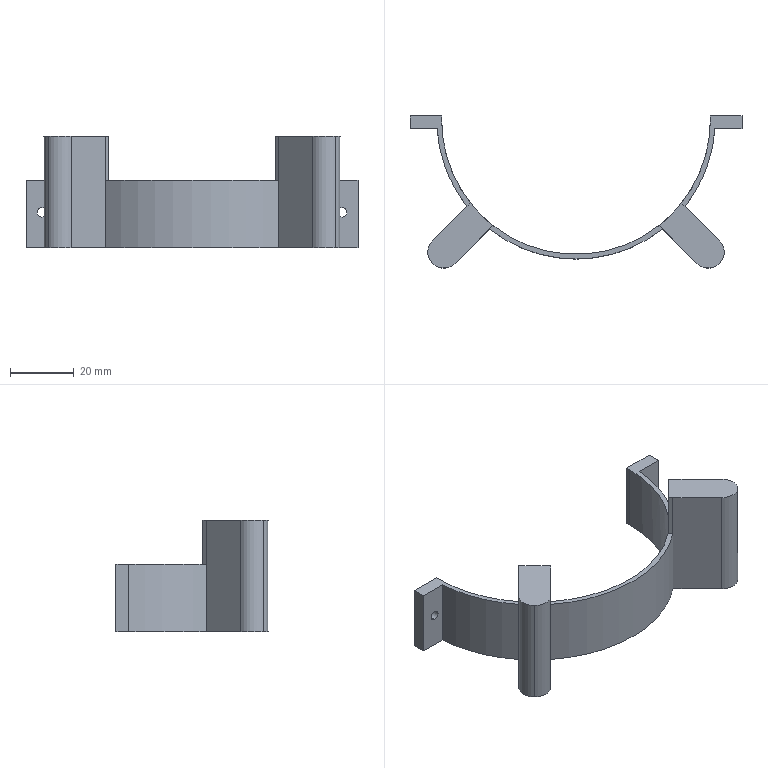Part | SolidWorks | features ICE 8, Fillet 2, CirPattern 1, Extrusion 1 | 1 solid | 40 faces | box 104 x 47.686 x 35 mm | volume 18349 mm3 | plane 22 | cylinder 18 | commonest cylinder face diameters 3 x4 5 x4 10 x4 84.2 x3 87.2 x3
STEP:
#1=CARTESIAN_POINT('',(43.936,-41.436,28.));
#2=VERTEX_POINT('',#1);
#3=CARTESIAN_POINT('',(38.936,-41.436,28.));
#4=VERTEX_POINT('',#3);
#5=CARTESIAN_POINT('',(41.436,-41.436,28.));
#6=DIRECTION('',(0.,0.,-1.));
#7=DIRECTION('',(0.,-1.,0.));
#8=AXIS2_PLACEMENT_3D('',#5,#6,#7);
#9=CIRCLE('',#8,2.5);
#10=EDGE_CURVE('',#2,#4,#9,.T.);
#11=ORIENTED_EDGE('',*,*,#10,.F.);
#12=CARTESIAN_POINT('',(43.936,-41.436,0.));
#13=VERTEX_POINT('',#12);
#14=CARTESIAN_POINT('',(43.936,-41.436,28.));
#15=DIRECTION('',(0.,0.,-1.));
#16=VECTOR('',#15,1000.);
#17=LINE('',#14,#16);
#18=EDGE_CURVE('',#2,#13,#17,.T.);
#19=ORIENTED_EDGE('',*,*,#18,.T.);
#20=CARTESIAN_POINT('',(38.936,-41.436,0.));
#21=VERTEX_POINT('',#20);
#22=CARTESIAN_POINT('',(41.436,-41.436,0.));
#23=DIRECTION('',(0.,0.,-1.));
#24=DIRECTION('',(0.,-1.,0.));
#25=AXIS2_PLACEMENT_3D('',#22,#23,#24);
#26=CIRCLE('',#25,2.5);
#27=EDGE_CURVE('',#13,#21,#26,.T.);
#28=ORIENTED_EDGE('',*,*,#27,.T.);
#29=CARTESIAN_POINT('',(38.936,-41.436,28.));
#30=DIRECTION('',(0.,0.,-1.));
#31=VECTOR('',#30,1000.);
#32=LINE('',#29,#31);
#33=EDGE_CURVE('',#4,#21,#32,.T.);
#34=ORIENTED_EDGE('',*,*,#33,.F.);
#35=EDGE_LOOP('',(#11,#19,#28,#34));
#36=FACE_OUTER_BOUND('',#35,.T.);
#37=CARTESIAN_POINT('',(41.436,-41.436,28.));
#38=DIRECTION('',(0.,0.,-1.));
#39=DIRECTION('',(-1.,0.,0.));
#40=AXIS2_PLACEMENT_3D('',#37,#38,#39);
#41=CYLINDRICAL_SURFACE('',#40,2.5);
#42=ADVANCED_FACE('',(#36),#41,.F.);
#43=CARTESIAN_POINT('',(-38.936,-41.436,28.));
#44=VERTEX_POINT('',#43);
#45=CARTESIAN_POINT('',(-43.936,-41.436,28.));
#46=VERTEX_POINT('',#45);
#47=CARTESIAN_POINT('',(-41.436,-41.436,28.));
#48=DIRECTION('',(0.,0.,-1.));
#49=DIRECTION('',(-1.,0.,0.));
#50=AXIS2_PLACEMENT_3D('',#47,#48,#49);
#51=CIRCLE('',#50,2.5);
#52=EDGE_CURVE('',#44,#46,#51,.T.);
#53=ORIENTED_EDGE('',*,*,#52,.F.);
#54=CARTESIAN_POINT('',(-38.936,-41.436,0.));
#55=VERTEX_POINT('',#54);
#56=CARTESIAN_POINT('',(-38.936,-41.436,28.));
#57=DIRECTION('',(0.,0.,-1.));
#58=VECTOR('',#57,1000.);
#59=LINE('',#56,#58);
#60=EDGE_CURVE('',#44,#55,#59,.T.);
#61=ORIENTED_EDGE('',*,*,#60,.T.);
#62=CARTESIAN_POINT('',(-43.936,-41.436,0.));
#63=VERTEX_POINT('',#62);
#64=CARTESIAN_POINT('',(-41.436,-41.436,0.));
#65=DIRECTION('',(0.,0.,-1.));
#66=DIRECTION('',(-1.,0.,0.));
#67=AXIS2_PLACEMENT_3D('',#64,#65,#66);
#68=CIRCLE('',#67,2.5);
#69=EDGE_CURVE('',#55,#63,#68,.T.);
#70=ORIENTED_EDGE('',*,*,#69,.T.);
#71=CARTESIAN_POINT('',(-43.936,-41.436,28.));
#72=DIRECTION('',(0.,0.,-1.));
#73=VECTOR('',#72,1000.);
#74=LINE('',#71,#73);
#75=EDGE_CURVE('',#46,#63,#74,.T.);
#76=ORIENTED_EDGE('',*,*,#75,.F.);
#77=EDGE_LOOP('',(#53,#61,#70,#76));
#78=FACE_OUTER_BOUND('',#77,.T.);
#79=CARTESIAN_POINT('',(-41.436,-41.436,28.));
#80=DIRECTION('',(0.,0.,-1.));
#81=DIRECTION('',(-1.,0.,0.));
#82=AXIS2_PLACEMENT_3D('',#79,#80,#81);
#83=CYLINDRICAL_SURFACE('',#82,2.5);
#84=ADVANCED_FACE('',(#78),#83,.F.);
#85=CARTESIAN_POINT('',(47.001,-2.75,9.64));
#86=VERTEX_POINT('',#85);
#87=CARTESIAN_POINT('',(47.001,-2.75,12.64));
#88=VERTEX_POINT('',#87);
#89=CARTESIAN_POINT('',(47.001,-2.75,11.14));
#90=DIRECTION('',(0.,1.,0.));
#91=DIRECTION('',(0.,0.,-1.));
#92=AXIS2_PLACEMENT_3D('',#89,#90,#91);
#93=CIRCLE('',#92,1.5);
#94=EDGE_CURVE('',#86,#88,#93,.T.);
#95=ORIENTED_EDGE('',*,*,#94,.F.);
#96=CARTESIAN_POINT('',(47.001,1.25,9.64));
#97=VERTEX_POINT('',#96);
#98=CARTESIAN_POINT('',(47.001,-43.601,9.64));
#99=DIRECTION('',(0.,1.,0.));
#100=VECTOR('',#99,1000.);
#101=LINE('',#98,#100);
#102=EDGE_CURVE('',#86,#97,#101,.T.);
#103=ORIENTED_EDGE('',*,*,#102,.T.);
#104=CARTESIAN_POINT('',(47.001,1.25,12.64));
#105=VERTEX_POINT('',#104);
#106=CARTESIAN_POINT('',(47.001,1.25,11.14));
#107=DIRECTION('',(0.,1.,0.));
#108=DIRECTION('',(0.,0.,1.));
#109=AXIS2_PLACEMENT_3D('',#106,#107,#108);
#110=CIRCLE('',#109,1.5);
#111=EDGE_CURVE('',#97,#105,#110,.T.);
#112=ORIENTED_EDGE('',*,*,#111,.T.);
#113=CARTESIAN_POINT('',(47.001,-43.601,12.64));
#114=DIRECTION('',(0.,1.,0.));
#115=VECTOR('',#114,1000.);
#116=LINE('',#113,#115);
#117=EDGE_CURVE('',#88,#105,#116,.T.);
#118=ORIENTED_EDGE('',*,*,#117,.F.);
#119=EDGE_LOOP('',(#95,#103,#112,#118));
#120=FACE_OUTER_BOUND('',#119,.T.);
#121=CARTESIAN_POINT('',(47.001,-43.601,11.14));
#122=DIRECTION('',(0.,1.,0.));
#123=DIRECTION('',(0.,0.,1.));
#124=AXIS2_PLACEMENT_3D('',#121,#122,#123);
#125=CYLINDRICAL_SURFACE('',#124,1.5);
#126=ADVANCED_FACE('',(#120),#125,.F.);
#127=CARTESIAN_POINT('',(-47.001,-2.75,12.64));
#128=VERTEX_POINT('',#127);
#129=CARTESIAN_POINT('',(-47.001,-2.75,9.64));
#130=VERTEX_POINT('',#129);
#131=CARTESIAN_POINT('',(-47.001,-2.75,11.14));
#132=DIRECTION('',(0.,-1.,0.));
#133=DIRECTION('',(0.,0.,1.));
#134=AXIS2_PLACEMENT_3D('',#131,#132,#133);
#135=CIRCLE('',#134,1.5);
#136=EDGE_CURVE('',#128,#130,#135,.T.);
#137=ORIENTED_EDGE('',*,*,#136,.T.);
#138=CARTESIAN_POINT('',(-47.001,1.25,9.64));
#139=VERTEX_POINT('',#138);
#140=CARTESIAN_POINT('',(-47.001,-43.601,9.64));
#141=DIRECTION('',(0.,1.,0.));
#142=VECTOR('',#141,1000.);
#143=LINE('',#140,#142);
#144=EDGE_CURVE('',#130,#139,#143,.T.);
#145=ORIENTED_EDGE('',*,*,#144,.T.);
#146=CARTESIAN_POINT('',(-47.001,1.25,12.64));
#147=VERTEX_POINT('',#146);
#148=CARTESIAN_POINT('',(-47.001,1.25,11.14));
#149=DIRECTION('',(0.,1.,0.));
#150=DIRECTION('',(0.,0.,1.));
#151=AXIS2_PLACEMENT_3D('',#148,#149,#150);
#152=CIRCLE('',#151,1.5);
#153=EDGE_CURVE('',#139,#147,#152,.T.);
#154=ORIENTED_EDGE('',*,*,#153,.T.);
#155=CARTESIAN_POINT('',(-47.001,-43.601,12.64));
#156=DIRECTION('',(0.,1.,0.));
#157=VECTOR('',#156,1000.);
#158=LINE('',#155,#157);
#159=EDGE_CURVE('',#128,#147,#158,.T.);
#160=ORIENTED_EDGE('',*,*,#159,.F.);
#161=EDGE_LOOP('',(#137,#145,#154,#160));
#162=FACE_OUTER_BOUND('',#161,.T.);
#163=CARTESIAN_POINT('',(-47.001,-43.601,11.14));
#164=DIRECTION('',(0.,1.,0.));
#165=DIRECTION('',(0.,0.,1.));
#166=AXIS2_PLACEMENT_3D('',#163,#164,#165);
#167=CYLINDRICAL_SURFACE('',#166,1.5);
#168=ADVANCED_FACE('',(#162),#167,.F.);
#169=CARTESIAN_POINT('',(33.094,-26.023,21.14));
#170=VERTEX_POINT('',#169);
#171=CARTESIAN_POINT('',(42.1,0.,21.14));
#172=VERTEX_POINT('',#171);
#173=CARTESIAN_POINT('',(0.,0.,21.14));
#174=DIRECTION('',(0.,0.,1.));
#175=DIRECTION('',(1.,0.,0.));
#176=AXIS2_PLACEMENT_3D('',#173,#174,#175);
#177=CIRCLE('',#176,42.1);
#178=EDGE_CURVE('',#170,#172,#177,.T.);
#179=ORIENTED_EDGE('',*,*,#178,.T.);
#180=CARTESIAN_POINT('',(42.1,0.,0.));
#181=VERTEX_POINT('',#180);
#182=CARTESIAN_POINT('',(42.1,0.,21.14));
#183=DIRECTION('',(0.,0.,-1.));
#184=VECTOR('',#183,1000.);
#185=LINE('',#182,#184);
#186=EDGE_CURVE('',#172,#181,#185,.T.);
#187=ORIENTED_EDGE('',*,*,#186,.T.);
#188=CARTESIAN_POINT('',(-42.1,0.,0.));
#189=VERTEX_POINT('',#188);
#190=CARTESIAN_POINT('',(0.,0.,0.));
#191=DIRECTION('',(0.,0.,1.));
#192=DIRECTION('',(1.,0.,0.));
#193=AXIS2_PLACEMENT_3D('',#190,#191,#192);
#194=CIRCLE('',#193,42.1);
#195=EDGE_CURVE('',#189,#181,#194,.T.);
#196=ORIENTED_EDGE('',*,*,#195,.F.);
#197=CARTESIAN_POINT('',(-42.1,0.,21.14));
#198=VERTEX_POINT('',#197);
#199=CARTESIAN_POINT('',(-42.1,0.,21.14));
#200=DIRECTION('',(0.,0.,-1.));
#201=VECTOR('',#200,1000.);
#202=LINE('',#199,#201);
#203=EDGE_CURVE('',#198,#189,#202,.T.);
#204=ORIENTED_EDGE('',*,*,#203,.F.);
#205=CARTESIAN_POINT('',(-33.098,-26.018,21.14));
#206=VERTEX_POINT('',#205);
#207=CARTESIAN_POINT('',(0.,0.,21.14));
#208=DIRECTION('',(0.,0.,1.));
#209=DIRECTION('',(1.,0.,0.));
#210=AXIS2_PLACEMENT_3D('',#207,#208,#209);
#211=CIRCLE('',#210,42.1);
#212=EDGE_CURVE('',#198,#206,#211,.T.);
#213=ORIENTED_EDGE('',*,*,#212,.T.);
#214=CARTESIAN_POINT('',(-33.098,-26.018,35.));
#215=VERTEX_POINT('',#214);
#216=CARTESIAN_POINT('',(-33.098,-26.018,35.));
#217=DIRECTION('',(0.,0.,-1.));
#218=VECTOR('',#217,1000.);
#219=LINE('',#216,#218);
#220=EDGE_CURVE('',#215,#206,#219,.T.);
#221=ORIENTED_EDGE('',*,*,#220,.F.);
#222=CARTESIAN_POINT('',(-26.023,-33.094,35.));
#223=VERTEX_POINT('',#222);
#224=CARTESIAN_POINT('',(0.,0.,35.));
#225=DIRECTION('',(0.,0.,-1.));
#226=DIRECTION('',(1.,0.,0.));
#227=AXIS2_PLACEMENT_3D('',#224,#225,#226);
#228=CIRCLE('',#227,42.1);
#229=EDGE_CURVE('',#223,#215,#228,.T.);
#230=ORIENTED_EDGE('',*,*,#229,.F.);
#231=CARTESIAN_POINT('',(-26.023,-33.094,21.14));
#232=VERTEX_POINT('',#231);
#233=CARTESIAN_POINT('',(-26.023,-33.094,35.));
#234=DIRECTION('',(0.,0.,-1.));
#235=VECTOR('',#234,1000.);
#236=LINE('',#233,#235);
#237=EDGE_CURVE('',#223,#232,#236,.T.);
#238=ORIENTED_EDGE('',*,*,#237,.T.);
#239=CARTESIAN_POINT('',(26.018,-33.098,21.14));
#240=VERTEX_POINT('',#239);
#241=CARTESIAN_POINT('',(0.,0.,21.14));
#242=DIRECTION('',(0.,0.,1.));
#243=DIRECTION('',(1.,0.,0.));
#244=AXIS2_PLACEMENT_3D('',#241,#242,#243);
#245=CIRCLE('',#244,42.1);
#246=EDGE_CURVE('',#232,#240,#245,.T.);
#247=ORIENTED_EDGE('',*,*,#246,.T.);
#248=CARTESIAN_POINT('',(26.018,-33.098,35.));
#249=VERTEX_POINT('',#248);
#250=CARTESIAN_POINT('',(26.018,-33.098,35.));
#251=DIRECTION('',(0.,0.,-1.));
#252=VECTOR('',#251,1000.);
#253=LINE('',#250,#252);
#254=EDGE_CURVE('',#249,#240,#253,.T.);
#255=ORIENTED_EDGE('',*,*,#254,.F.);
#256=CARTESIAN_POINT('',(33.094,-26.023,35.));
#257=VERTEX_POINT('',#256);
#258=CARTESIAN_POINT('',(0.,0.,35.));
#259=DIRECTION('',(0.,0.,-1.));
#260=DIRECTION('',(0.,1.,0.));
#261=AXIS2_PLACEMENT_3D('',#258,#259,#260);
#262=CIRCLE('',#261,42.1);
#263=EDGE_CURVE('',#257,#249,#262,.T.);
#264=ORIENTED_EDGE('',*,*,#263,.F.);
#265=CARTESIAN_POINT('',(33.094,-26.023,35.));
#266=DIRECTION('',(0.,0.,-1.));
#267=VECTOR('',#266,1000.);
#268=LINE('',#265,#267);
#269=EDGE_CURVE('',#257,#170,#268,.T.);
#270=ORIENTED_EDGE('',*,*,#269,.T.);
#271=EDGE_LOOP('',(#179,#187,#196,#204,#213,#221,#230,#238,#247,#255,#264,#270));
#272=FACE_OUTER_BOUND('',#271,.T.);
#273=CARTESIAN_POINT('',(0.,0.,21.14));
#274=DIRECTION('',(0.,0.,-1.));
#275=DIRECTION('',(-1.,0.,0.));
#276=AXIS2_PLACEMENT_3D('',#273,#274,#275);
#277=CYLINDRICAL_SURFACE('',#276,42.1);
#278=ADVANCED_FACE('',(#272),#277,.F.);
#279=CARTESIAN_POINT('',(-42.081,1.25,21.14));
#280=VERTEX_POINT('',#279);
#281=CARTESIAN_POINT('',(0.,0.,21.14));
#282=DIRECTION('',(0.,0.,1.));
#283=DIRECTION('',(1.,0.,0.));
#284=AXIS2_PLACEMENT_3D('',#281,#282,#283);
#285=CIRCLE('',#284,42.1);
#286=EDGE_CURVE('',#280,#198,#285,.T.);
#287=ORIENTED_EDGE('',*,*,#286,.T.);
#288=ORIENTED_EDGE('',*,*,#203,.T.);
#289=CARTESIAN_POINT('',(-42.081,1.25,0.));
#290=VERTEX_POINT('',#289);
#291=CARTESIAN_POINT('',(0.,0.,0.));
#292=DIRECTION('',(0.,0.,1.));
#293=DIRECTION('',(1.,0.,0.));
#294=AXIS2_PLACEMENT_3D('',#291,#292,#293);
#295=CIRCLE('',#294,42.1);
#296=EDGE_CURVE('',#290,#189,#295,.T.);
#297=ORIENTED_EDGE('',*,*,#296,.F.);
#298=CARTESIAN_POINT('',(-42.081,1.25,21.14));
#299=DIRECTION('',(0.,0.,-1.));
#300=VECTOR('',#299,1000.);
#301=LINE('',#298,#300);
#302=EDGE_CURVE('',#280,#290,#301,.T.);
#303=ORIENTED_EDGE('',*,*,#302,.F.);
#304=EDGE_LOOP('',(#287,#288,#297,#303));
#305=FACE_OUTER_BOUND('',#304,.T.);
#306=CARTESIAN_POINT('',(0.,0.,21.14));
#307=DIRECTION('',(0.,0.,-1.));
#308=DIRECTION('',(-1.,0.,0.));
#309=AXIS2_PLACEMENT_3D('',#306,#307,#308);
#310=CYLINDRICAL_SURFACE('',#309,42.1);
#311=ADVANCED_FACE('',(#305),#310,.F.);
#312=CARTESIAN_POINT('',(-27.091,-34.162,21.14));
#313=VERTEX_POINT('',#312);
#314=CARTESIAN_POINT('',(27.091,-34.162,21.14));
#315=VERTEX_POINT('',#314);
#316=CARTESIAN_POINT('',(0.,0.,21.14));
#317=DIRECTION('',(0.,0.,1.));
#318=DIRECTION('',(1.,0.,0.));
#319=AXIS2_PLACEMENT_3D('',#316,#317,#318);
#320=CIRCLE('',#319,43.6);
#321=EDGE_CURVE('',#313,#315,#320,.T.);
#322=ORIENTED_EDGE('',*,*,#321,.T.);
#323=CARTESIAN_POINT('',(26.018,-33.098,21.14));
#324=DIRECTION('',(0.7098,-0.7044,0.));
#325=VECTOR('',#324,1000.);
#326=LINE('',#323,#325);
#327=EDGE_CURVE('',#240,#315,#326,.T.);
#328=ORIENTED_EDGE('',*,*,#327,.F.);
#329=ORIENTED_EDGE('',*,*,#246,.F.);
#330=CARTESIAN_POINT('',(-26.023,-33.094,21.14));
#331=DIRECTION('',(0.7068,0.7074,0.));
#332=VECTOR('',#331,1000.);
#333=LINE('',#330,#332);
#334=EDGE_CURVE('',#313,#232,#333,.T.);
#335=ORIENTED_EDGE('',*,*,#334,.F.);
#336=EDGE_LOOP('',(#322,#328,#329,#335));
#337=FACE_OUTER_BOUND('',#336,.T.);
#338=CARTESIAN_POINT('',(0.,0.,21.14));
#339=DIRECTION('',(0.,0.,1.));
#340=DIRECTION('',(1.,0.,0.));
#341=AXIS2_PLACEMENT_3D('',#338,#339,#340);
#342=PLANE('',#341);
#343=ADVANCED_FACE('',(#337),#342,.T.);
#344=ORIENTED_EDGE('',*,*,#178,.F.);
#345=CARTESIAN_POINT('',(34.162,-27.091,21.14));
#346=VERTEX_POINT('',#345);
#347=CARTESIAN_POINT('',(33.094,-26.023,21.14));
#348=DIRECTION('',(-0.7074,0.7068,0.));
#349=VECTOR('',#348,1000.);
#350=LINE('',#347,#349);
#351=EDGE_CURVE('',#346,#170,#350,.T.);
#352=ORIENTED_EDGE('',*,*,#351,.F.);
#353=CARTESIAN_POINT('',(43.513,-2.75,21.14));
#354=VERTEX_POINT('',#353);
#355=CARTESIAN_POINT('',(0.,0.,21.14));
#356=DIRECTION('',(0.,0.,1.));
#357=DIRECTION('',(1.,0.,0.));
#358=AXIS2_PLACEMENT_3D('',#355,#356,#357);
#359=CIRCLE('',#358,43.6);
#360=EDGE_CURVE('',#346,#354,#359,.T.);
#361=ORIENTED_EDGE('',*,*,#360,.T.);
#362=CARTESIAN_POINT('',(52.,-2.75,21.14));
#363=VERTEX_POINT('',#362);
#364=CARTESIAN_POINT('',(-52.002,-2.75,21.14));
#365=DIRECTION('',(1.,0.,0.));
#366=VECTOR('',#365,1000.);
#367=LINE('',#364,#366);
#368=EDGE_CURVE('',#354,#363,#367,.T.);
#369=ORIENTED_EDGE('',*,*,#368,.T.);
#370=CARTESIAN_POINT('',(52.,1.25,21.14));
#371=VERTEX_POINT('',#370);
#372=CARTESIAN_POINT('',(52.,1.25,21.14));
#373=DIRECTION('',(0.,-1.,0.));
#374=VECTOR('',#373,1000.);
#375=LINE('',#372,#374);
#376=EDGE_CURVE('',#371,#363,#375,.T.);
#377=ORIENTED_EDGE('',*,*,#376,.F.);
#378=CARTESIAN_POINT('',(42.081,1.25,21.14));
#379=VERTEX_POINT('',#378);
#380=CARTESIAN_POINT('',(0.,1.25,21.14));
#381=DIRECTION('',(1.,0.,0.));
#382=VECTOR('',#381,1000.);
#383=LINE('',#380,#382);
#384=EDGE_CURVE('',#379,#371,#383,.T.);
#385=ORIENTED_EDGE('',*,*,#384,.F.);
#386=CARTESIAN_POINT('',(0.,0.,21.14));
#387=DIRECTION('',(0.,0.,1.));
#388=DIRECTION('',(1.,0.,0.));
#389=AXIS2_PLACEMENT_3D('',#386,#387,#388);
#390=CIRCLE('',#389,42.1);
#391=EDGE_CURVE('',#172,#379,#390,.T.);
#392=ORIENTED_EDGE('',*,*,#391,.F.);
#393=EDGE_LOOP('',(#344,#352,#361,#369,#377,#385,#392));
#394=FACE_OUTER_BOUND('',#393,.T.);
#395=CARTESIAN_POINT('',(0.,0.,21.14));
#396=DIRECTION('',(0.,0.,1.));
#397=DIRECTION('',(1.,0.,0.));
#398=AXIS2_PLACEMENT_3D('',#395,#396,#397);
#399=PLANE('',#398);
#400=ADVANCED_FACE('',(#394),#399,.T.);
#401=CARTESIAN_POINT('',(27.091,-34.162,0.));
#402=VERTEX_POINT('',#401);
#403=CARTESIAN_POINT('',(27.091,-34.162,21.14));
#404=DIRECTION('',(0.,0.,1.));
#405=VECTOR('',#404,1000.);
#406=LINE('',#403,#405);
#407=EDGE_CURVE('',#402,#315,#406,.T.);
#408=ORIENTED_EDGE('',*,*,#407,.T.);
#409=ORIENTED_EDGE('',*,*,#321,.F.);
#410=CARTESIAN_POINT('',(-27.091,-34.162,0.));
#411=VERTEX_POINT('',#410);
#412=CARTESIAN_POINT('',(-27.091,-34.162,21.14));
#413=DIRECTION('',(0.,0.,-1.));
#414=VECTOR('',#413,1000.);
#415=LINE('',#412,#414);
#416=EDGE_CURVE('',#313,#411,#415,.T.);
#417=ORIENTED_EDGE('',*,*,#416,.T.);
#418=CARTESIAN_POINT('',(0.,0.,0.));
#419=DIRECTION('',(0.,0.,1.));
#420=DIRECTION('',(1.,0.,0.));
#421=AXIS2_PLACEMENT_3D('',#418,#419,#420);
#422=CIRCLE('',#421,43.6);
#423=EDGE_CURVE('',#411,#402,#422,.T.);
#424=ORIENTED_EDGE('',*,*,#423,.T.);
#425=EDGE_LOOP('',(#408,#409,#417,#424));
#426=FACE_OUTER_BOUND('',#425,.T.);
#427=CARTESIAN_POINT('',(0.,0.,21.14));
#428=DIRECTION('',(0.,0.,-1.));
#429=DIRECTION('',(-1.,0.,0.));
#430=AXIS2_PLACEMENT_3D('',#427,#428,#429);
#431=CYLINDRICAL_SURFACE('',#430,43.6);
#432=ADVANCED_FACE('',(#426),#431,.T.);
#433=CARTESIAN_POINT('',(34.162,-27.091,0.));
#434=VERTEX_POINT('',#433);
#435=CARTESIAN_POINT('',(34.162,-27.091,21.14));
#436=DIRECTION('',(0.,0.,-1.));
#437=VECTOR('',#436,1000.);
#438=LINE('',#435,#437);
#439=EDGE_CURVE('',#346,#434,#438,.T.);
#440=ORIENTED_EDGE('',*,*,#439,.T.);
#441=CARTESIAN_POINT('',(43.513,-2.75,0.));
#442=VERTEX_POINT('',#441);
#443=CARTESIAN_POINT('',(0.,0.,0.));
#444=DIRECTION('',(0.,0.,1.));
#445=DIRECTION('',(1.,0.,0.));
#446=AXIS2_PLACEMENT_3D('',#443,#444,#445);
#447=CIRCLE('',#446,43.6);
#448=EDGE_CURVE('',#434,#442,#447,.T.);
#449=ORIENTED_EDGE('',*,*,#448,.T.);
#450=CARTESIAN_POINT('',(43.513,-2.75,21.14));
#451=DIRECTION('',(0.,0.,-1.));
#452=VECTOR('',#451,1000.);
#453=LINE('',#450,#452);
#454=EDGE_CURVE('',#354,#442,#453,.T.);
#455=ORIENTED_EDGE('',*,*,#454,.F.);
#456=ORIENTED_EDGE('',*,*,#360,.F.);
#457=EDGE_LOOP('',(#440,#449,#455,#456));
#458=FACE_OUTER_BOUND('',#457,.T.);
#459=CARTESIAN_POINT('',(0.,0.,21.14));
#460=DIRECTION('',(0.,0.,-1.));
#461=DIRECTION('',(-1.,0.,0.));
#462=AXIS2_PLACEMENT_3D('',#459,#460,#461);
#463=CYLINDRICAL_SURFACE('',#462,43.6);
#464=ADVANCED_FACE('',(#458),#463,.T.);
#465=CARTESIAN_POINT('',(-34.162,-27.091,0.));
#466=VERTEX_POINT('',#465);
#467=CARTESIAN_POINT('',(-34.162,-27.091,21.14));
#468=VERTEX_POINT('',#467);
#469=CARTESIAN_POINT('',(-34.162,-27.091,21.14));
#470=DIRECTION('',(0.,0.,1.));
#471=VECTOR('',#470,1000.);
#472=LINE('',#469,#471);
#473=EDGE_CURVE('',#466,#468,#472,.T.);
#474=ORIENTED_EDGE('',*,*,#473,.T.);
#475=CARTESIAN_POINT('',(-43.513,-2.75,21.14));
#476=VERTEX_POINT('',#475);
#477=CARTESIAN_POINT('',(0.,0.,21.14));
#478=DIRECTION('',(0.,0.,1.));
#479=DIRECTION('',(1.,0.,0.));
#480=AXIS2_PLACEMENT_3D('',#477,#478,#479);
#481=CIRCLE('',#480,43.6);
#482=EDGE_CURVE('',#476,#468,#481,.T.);
#483=ORIENTED_EDGE('',*,*,#482,.F.);
#484=CARTESIAN_POINT('',(-43.513,-2.75,0.));
#485=VERTEX_POINT('',#484);
#486=CARTESIAN_POINT('',(-43.513,-2.75,21.14));
#487=DIRECTION('',(0.,0.,-1.));
#488=VECTOR('',#487,1000.);
#489=LINE('',#486,#488);
#490=EDGE_CURVE('',#476,#485,#489,.T.);
#491=ORIENTED_EDGE('',*,*,#490,.T.);
#492=CARTESIAN_POINT('',(0.,0.,0.));
#493=DIRECTION('',(0.,0.,1.));
#494=DIRECTION('',(1.,0.,0.));
#495=AXIS2_PLACEMENT_3D('',#492,#493,#494);
#496=CIRCLE('',#495,43.6);
#497=EDGE_CURVE('',#485,#466,#496,.T.);
#498=ORIENTED_EDGE('',*,*,#497,.T.);
#499=EDGE_LOOP('',(#474,#483,#491,#498));
#500=FACE_OUTER_BOUND('',#499,.T.);
#501=CARTESIAN_POINT('',(0.,0.,21.14));
#502=DIRECTION('',(0.,0.,-1.));
#503=DIRECTION('',(-1.,0.,0.));
#504=AXIS2_PLACEMENT_3D('',#501,#502,#503);
#505=CYLINDRICAL_SURFACE('',#504,43.6);
#506=ADVANCED_FACE('',(#500),#505,.T.);
#507=CARTESIAN_POINT('',(-33.098,-26.018,21.14));
#508=DIRECTION('',(-0.7044,-0.7098,0.));
#509=VECTOR('',#508,1000.);
#510=LINE('',#507,#509);
#511=EDGE_CURVE('',#206,#468,#510,.T.);
#512=ORIENTED_EDGE('',*,*,#511,.F.);
#513=ORIENTED_EDGE('',*,*,#212,.F.);
#514=ORIENTED_EDGE('',*,*,#286,.F.);
#515=CARTESIAN_POINT('',(-52.,1.25,21.14));
#516=VERTEX_POINT('',#515);
#517=CARTESIAN_POINT('',(0.,1.25,21.14));
#518=DIRECTION('',(1.,0.,0.));
#519=VECTOR('',#518,1000.);
#520=LINE('',#517,#519);
#521=EDGE_CURVE('',#516,#280,#520,.T.);
#522=ORIENTED_EDGE('',*,*,#521,.F.);
#523=CARTESIAN_POINT('',(-52.,-2.75,21.14));
#524=VERTEX_POINT('',#523);
#525=CARTESIAN_POINT('',(-52.,1.25,21.14));
#526=DIRECTION('',(0.,-1.,0.));
#527=VECTOR('',#526,1000.);
#528=LINE('',#525,#527);
#529=EDGE_CURVE('',#516,#524,#528,.T.);
#530=ORIENTED_EDGE('',*,*,#529,.T.);
#531=CARTESIAN_POINT('',(43.602,-2.75,21.14));
#532=DIRECTION('',(-1.,0.,0.));
#533=VECTOR('',#532,1000.);
#534=LINE('',#531,#533);
#535=EDGE_CURVE('',#476,#524,#534,.T.);
#536=ORIENTED_EDGE('',*,*,#535,.F.);
#537=ORIENTED_EDGE('',*,*,#482,.T.);
#538=EDGE_LOOP('',(#512,#513,#514,#522,#530,#536,#537));
#539=FACE_OUTER_BOUND('',#538,.T.);
#540=CARTESIAN_POINT('',(0.,0.,21.14));
#541=DIRECTION('',(0.,0.,1.));
#542=DIRECTION('',(1.,0.,0.));
#543=AXIS2_PLACEMENT_3D('',#540,#541,#542);
#544=PLANE('',#543);
#545=ADVANCED_FACE('',(#539),#544,.T.);
#546=CARTESIAN_POINT('',(41.436,-41.436,0.));
#547=DIRECTION('',(0.,0.,-1.));
#548=DIRECTION('',(0.,-1.,0.));
#549=AXIS2_PLACEMENT_3D('',#546,#547,#548);
#550=CIRCLE('',#549,2.5);
#551=EDGE_CURVE('',#21,#13,#550,.T.);
#552=ORIENTED_EDGE('',*,*,#551,.F.);
#553=ORIENTED_EDGE('',*,*,#27,.F.);
#554=EDGE_LOOP('',(#552,#553));
#555=FACE_BOUND('',#554,.T.);
#556=CARTESIAN_POINT('',(-41.436,-41.436,0.));
#557=DIRECTION('',(0.,0.,-1.));
#558=DIRECTION('',(-1.,0.,0.));
#559=AXIS2_PLACEMENT_3D('',#556,#557,#558);
#560=CIRCLE('',#559,2.5);
#561=EDGE_CURVE('',#63,#55,#560,.T.);
#562=ORIENTED_EDGE('',*,*,#561,.F.);
#563=ORIENTED_EDGE('',*,*,#69,.F.);
#564=EDGE_LOOP('',(#562,#563));
#565=FACE_BOUND('',#564,.T.);
#566=CARTESIAN_POINT('',(-37.901,-44.972,0.));
#567=VERTEX_POINT('',#566);
#568=CARTESIAN_POINT('',(-44.972,-44.972,0.));
#569=VERTEX_POINT('',#568);
#570=CARTESIAN_POINT('',(-41.436,-41.436,0.));
#571=DIRECTION('',(0.,0.,-1.));
#572=DIRECTION('',(1.,0.,0.));
#573=AXIS2_PLACEMENT_3D('',#570,#571,#572);
#574=CIRCLE('',#573,5.);
#575=EDGE_CURVE('',#567,#569,#574,.T.);
#576=ORIENTED_EDGE('',*,*,#575,.T.);
#577=CARTESIAN_POINT('',(-44.972,-37.901,0.));
#578=VERTEX_POINT('',#577);
#579=CARTESIAN_POINT('',(-41.436,-41.436,0.));
#580=DIRECTION('',(0.,0.,-1.));
#581=DIRECTION('',(1.,0.,0.));
#582=AXIS2_PLACEMENT_3D('',#579,#580,#581);
#583=CIRCLE('',#582,5.);
#584=EDGE_CURVE('',#569,#578,#583,.T.);
#585=ORIENTED_EDGE('',*,*,#584,.T.);
#586=CARTESIAN_POINT('',(23.091,30.162,0.));
#587=DIRECTION('',(-0.7071,-0.7071,0.));
#588=VECTOR('',#587,1000.);
#589=LINE('',#586,#588);
#590=EDGE_CURVE('',#466,#578,#589,.T.);
#591=ORIENTED_EDGE('',*,*,#590,.F.);
#592=ORIENTED_EDGE('',*,*,#497,.F.);
#593=CARTESIAN_POINT('',(-52.,-2.75,0.));
#594=VERTEX_POINT('',#593);
#595=CARTESIAN_POINT('',(43.602,-2.75,0.));
#596=DIRECTION('',(-1.,0.,0.));
#597=VECTOR('',#596,1000.);
#598=LINE('',#595,#597);
#599=EDGE_CURVE('',#485,#594,#598,.T.);
#600=ORIENTED_EDGE('',*,*,#599,.T.);
#601=CARTESIAN_POINT('',(-52.,1.25,0.));
#602=VERTEX_POINT('',#601);
#603=CARTESIAN_POINT('',(-52.,1.25,0.));
#604=DIRECTION('',(0.,1.,0.));
#605=VECTOR('',#604,1000.);
#606=LINE('',#603,#605);
#607=EDGE_CURVE('',#594,#602,#606,.T.);
#608=ORIENTED_EDGE('',*,*,#607,.T.);
#609=CARTESIAN_POINT('',(0.,1.25,0.));
#610=DIRECTION('',(1.,0.,0.));
#611=VECTOR('',#610,1000.);
#612=LINE('',#609,#611);
#613=EDGE_CURVE('',#602,#290,#612,.T.);
#614=ORIENTED_EDGE('',*,*,#613,.T.);
#615=ORIENTED_EDGE('',*,*,#296,.T.);
#616=ORIENTED_EDGE('',*,*,#195,.T.);
#617=CARTESIAN_POINT('',(42.081,1.25,0.));
#618=VERTEX_POINT('',#617);
#619=CARTESIAN_POINT('',(0.,0.,0.));
#620=DIRECTION('',(0.,0.,1.));
#621=DIRECTION('',(1.,0.,0.));
#622=AXIS2_PLACEMENT_3D('',#619,#620,#621);
#623=CIRCLE('',#622,42.1);
#624=EDGE_CURVE('',#181,#618,#623,.T.);
#625=ORIENTED_EDGE('',*,*,#624,.T.);
#626=CARTESIAN_POINT('',(52.,1.25,0.));
#627=VERTEX_POINT('',#626);
#628=CARTESIAN_POINT('',(0.,1.25,0.));
#629=DIRECTION('',(1.,0.,0.));
#630=VECTOR('',#629,1000.);
#631=LINE('',#628,#630);
#632=EDGE_CURVE('',#618,#627,#631,.T.);
#633=ORIENTED_EDGE('',*,*,#632,.T.);
#634=CARTESIAN_POINT('',(52.,-2.75,0.));
#635=VERTEX_POINT('',#634);
#636=CARTESIAN_POINT('',(52.,1.25,0.));
#637=DIRECTION('',(0.,1.,0.));
#638=VECTOR('',#637,1000.);
#639=LINE('',#636,#638);
#640=EDGE_CURVE('',#635,#627,#639,.T.);
#641=ORIENTED_EDGE('',*,*,#640,.F.);
#642=CARTESIAN_POINT('',(-52.002,-2.75,0.));
#643=DIRECTION('',(1.,0.,0.));
#644=VECTOR('',#643,1000.);
#645=LINE('',#642,#644);
#646=EDGE_CURVE('',#442,#635,#645,.T.);
#647=ORIENTED_EDGE('',*,*,#646,.F.);
#648=ORIENTED_EDGE('',*,*,#448,.F.);
#649=CARTESIAN_POINT('',(44.972,-37.901,0.));
#650=VERTEX_POINT('',#649);
#651=CARTESIAN_POINT('',(-23.091,30.162,0.));
#652=DIRECTION('',(0.7071,-0.7071,0.));
#653=VECTOR('',#652,1000.);
#654=LINE('',#651,#653);
#655=EDGE_CURVE('',#434,#650,#654,.T.);
#656=ORIENTED_EDGE('',*,*,#655,.T.);
#657=CARTESIAN_POINT('',(44.972,-44.972,0.));
#658=VERTEX_POINT('',#657);
#659=CARTESIAN_POINT('',(41.436,-41.436,0.));
#660=DIRECTION('',(0.,0.,-1.));
#661=DIRECTION('',(1.,0.,0.));
#662=AXIS2_PLACEMENT_3D('',#659,#660,#661);
#663=CIRCLE('',#662,5.);
#664=EDGE_CURVE('',#650,#658,#663,.T.);
#665=ORIENTED_EDGE('',*,*,#664,.T.);
#666=CARTESIAN_POINT('',(37.901,-44.972,0.));
#667=VERTEX_POINT('',#666);
#668=CARTESIAN_POINT('',(41.436,-41.436,0.));
#669=DIRECTION('',(0.,0.,-1.));
#670=DIRECTION('',(1.,0.,0.));
#671=AXIS2_PLACEMENT_3D('',#668,#669,#670);
#672=CIRCLE('',#671,5.);
#673=EDGE_CURVE('',#658,#667,#672,.T.);
#674=ORIENTED_EDGE('',*,*,#673,.T.);
#675=CARTESIAN_POINT('',(-30.162,23.091,0.));
#676=DIRECTION('',(0.7071,-0.7071,0.));
#677=VECTOR('',#676,1000.);
#678=LINE('',#675,#677);
#679=EDGE_CURVE('',#402,#667,#678,.T.);
#680=ORIENTED_EDGE('',*,*,#679,.F.);
#681=ORIENTED_EDGE('',*,*,#423,.F.);
#682=CARTESIAN_POINT('',(30.162,23.091,0.));
#683=DIRECTION('',(-0.7071,-0.7071,0.));
#684=VECTOR('',#683,1000.);
#685=LINE('',#682,#684);
#686=EDGE_CURVE('',#411,#567,#685,.T.);
#687=ORIENTED_EDGE('',*,*,#686,.T.);
#688=EDGE_LOOP('',(#576,#585,#591,#592,#600,#608,#614,#615,#616,#625,#633,#641,#647,#648,#656,#665,#674,#680,#681,#687));
#689=FACE_OUTER_BOUND('',#688,.T.);
#690=CARTESIAN_POINT('',(0.,0.,0.));
#691=DIRECTION('',(0.,0.,1.));
#692=DIRECTION('',(1.,0.,0.));
#693=AXIS2_PLACEMENT_3D('',#690,#691,#692);
#694=PLANE('',#693);
#695=ADVANCED_FACE('',(#555,#565,#689),#694,.F.);
#696=ORIENTED_EDGE('',*,*,#186,.F.);
#697=ORIENTED_EDGE('',*,*,#391,.T.);
#698=CARTESIAN_POINT('',(42.081,1.25,21.14));
#699=DIRECTION('',(0.,0.,1.));
#700=VECTOR('',#699,1000.);
#701=LINE('',#698,#700);
#702=EDGE_CURVE('',#618,#379,#701,.T.);
#703=ORIENTED_EDGE('',*,*,#702,.F.);
#704=ORIENTED_EDGE('',*,*,#624,.F.);
#705=EDGE_LOOP('',(#696,#697,#703,#704));
#706=FACE_OUTER_BOUND('',#705,.T.);
#707=CARTESIAN_POINT('',(0.,0.,21.14));
#708=DIRECTION('',(0.,0.,-1.));
#709=DIRECTION('',(-1.,0.,0.));
#710=AXIS2_PLACEMENT_3D('',#707,#708,#709);
#711=CYLINDRICAL_SURFACE('',#710,42.1);
#712=ADVANCED_FACE('',(#706),#711,.F.);
#713=CARTESIAN_POINT('',(47.001,1.25,11.14));
#714=DIRECTION('',(0.,1.,0.));
#715=DIRECTION('',(0.,0.,1.));
#716=AXIS2_PLACEMENT_3D('',#713,#714,#715);
#717=CIRCLE('',#716,1.5);
#718=EDGE_CURVE('',#105,#97,#717,.T.);
#719=ORIENTED_EDGE('',*,*,#718,.F.);
#720=ORIENTED_EDGE('',*,*,#111,.F.);
#721=EDGE_LOOP('',(#719,#720));
#722=FACE_BOUND('',#721,.T.);
#723=ORIENTED_EDGE('',*,*,#632,.F.);
#724=ORIENTED_EDGE('',*,*,#702,.T.);
#725=ORIENTED_EDGE('',*,*,#384,.T.);
#726=CARTESIAN_POINT('',(52.,1.25,0.));
#727=DIRECTION('',(0.,0.,1.));
#728=VECTOR('',#727,1000.);
#729=LINE('',#726,#728);
#730=EDGE_CURVE('',#627,#371,#729,.T.);
#731=ORIENTED_EDGE('',*,*,#730,.F.);
#732=EDGE_LOOP('',(#723,#724,#725,#731));
#733=FACE_OUTER_BOUND('',#732,.T.);
#734=CARTESIAN_POINT('',(0.,1.25,0.));
#735=DIRECTION('',(0.,1.,0.));
#736=DIRECTION('',(0.,0.,1.));
#737=AXIS2_PLACEMENT_3D('',#734,#735,#736);
#738=PLANE('',#737);
#739=ADVANCED_FACE('',(#722,#733),#738,.T.);
#740=CARTESIAN_POINT('',(-47.001,1.25,11.14));
#741=DIRECTION('',(0.,1.,0.));
#742=DIRECTION('',(0.,0.,1.));
#743=AXIS2_PLACEMENT_3D('',#740,#741,#742);
#744=CIRCLE('',#743,1.5);
#745=EDGE_CURVE('',#147,#139,#744,.T.);
#746=ORIENTED_EDGE('',*,*,#745,.F.);
#747=ORIENTED_EDGE('',*,*,#153,.F.);
#748=EDGE_LOOP('',(#746,#747));
#749=FACE_BOUND('',#748,.T.);
#750=ORIENTED_EDGE('',*,*,#521,.T.);
#751=ORIENTED_EDGE('',*,*,#302,.T.);
#752=ORIENTED_EDGE('',*,*,#613,.F.);
#753=CARTESIAN_POINT('',(-52.,1.25,21.14));
#754=DIRECTION('',(0.,0.,1.));
#755=VECTOR('',#754,1000.);
#756=LINE('',#753,#755);
#757=EDGE_CURVE('',#602,#516,#756,.T.);
#758=ORIENTED_EDGE('',*,*,#757,.T.);
#759=EDGE_LOOP('',(#750,#751,#752,#758));
#760=FACE_OUTER_BOUND('',#759,.T.);
#761=CARTESIAN_POINT('',(0.,1.25,0.));
#762=DIRECTION('',(0.,1.,0.));
#763=DIRECTION('',(0.,0.,1.));
#764=AXIS2_PLACEMENT_3D('',#761,#762,#763);
#765=PLANE('',#764);
#766=ADVANCED_FACE('',(#749,#760),#765,.T.);
#767=ORIENTED_EDGE('',*,*,#529,.F.);
#768=ORIENTED_EDGE('',*,*,#757,.F.);
#769=ORIENTED_EDGE('',*,*,#607,.F.);
#770=CARTESIAN_POINT('',(-52.,-2.75,21.14));
#771=DIRECTION('',(0.,0.,-1.));
#772=VECTOR('',#771,1000.);
#773=LINE('',#770,#772);
#774=EDGE_CURVE('',#524,#594,#773,.T.);
#775=ORIENTED_EDGE('',*,*,#774,.F.);
#776=EDGE_LOOP('',(#767,#768,#769,#775));
#777=FACE_OUTER_BOUND('',#776,.T.);
#778=CARTESIAN_POINT('',(-52.,0.,0.));
#779=DIRECTION('',(1.,0.,0.));
#780=DIRECTION('',(0.,0.,-1.));
#781=AXIS2_PLACEMENT_3D('',#778,#779,#780);
#782=PLANE('',#781);
#783=ADVANCED_FACE('',(#777),#782,.F.);
#784=ORIENTED_EDGE('',*,*,#136,.F.);
#785=CARTESIAN_POINT('',(-47.001,-2.75,11.14));
#786=DIRECTION('',(0.,-1.,0.));
#787=DIRECTION('',(0.,0.,1.));
#788=AXIS2_PLACEMENT_3D('',#785,#786,#787);
#789=CIRCLE('',#788,1.5);
#790=EDGE_CURVE('',#130,#128,#789,.T.);
#791=ORIENTED_EDGE('',*,*,#790,.F.);
#792=EDGE_LOOP('',(#784,#791));
#793=FACE_BOUND('',#792,.T.);
#794=ORIENTED_EDGE('',*,*,#490,.F.);
#795=ORIENTED_EDGE('',*,*,#535,.T.);
#796=ORIENTED_EDGE('',*,*,#774,.T.);
#797=ORIENTED_EDGE('',*,*,#599,.F.);
#798=EDGE_LOOP('',(#794,#795,#796,#797));
#799=FACE_OUTER_BOUND('',#798,.T.);
#800=CARTESIAN_POINT('',(43.602,-2.75,21.14));
#801=DIRECTION('',(0.,1.,0.));
#802=DIRECTION('',(0.,0.,1.));
#803=AXIS2_PLACEMENT_3D('',#800,#801,#802);
#804=PLANE('',#803);
#805=ADVANCED_FACE('',(#793,#799),#804,.F.);
#806=ORIENTED_EDGE('',*,*,#144,.F.);
#807=ORIENTED_EDGE('',*,*,#790,.T.);
#808=ORIENTED_EDGE('',*,*,#159,.T.);
#809=ORIENTED_EDGE('',*,*,#745,.T.);
#810=EDGE_LOOP('',(#806,#807,#808,#809));
#811=FACE_OUTER_BOUND('',#810,.T.);
#812=CARTESIAN_POINT('',(-47.001,-43.601,11.14));
#813=DIRECTION('',(0.,1.,0.));
#814=DIRECTION('',(0.,0.,1.));
#815=AXIS2_PLACEMENT_3D('',#812,#813,#814);
#816=CYLINDRICAL_SURFACE('',#815,1.5);
#817=ADVANCED_FACE('',(#811),#816,.F.);
#818=ORIENTED_EDGE('',*,*,#640,.T.);
#819=ORIENTED_EDGE('',*,*,#730,.T.);
#820=ORIENTED_EDGE('',*,*,#376,.T.);
#821=CARTESIAN_POINT('',(52.,-2.75,0.));
#822=DIRECTION('',(0.,0.,-1.));
#823=VECTOR('',#822,1000.);
#824=LINE('',#821,#823);
#825=EDGE_CURVE('',#363,#635,#824,.T.);
#826=ORIENTED_EDGE('',*,*,#825,.T.);
#827=EDGE_LOOP('',(#818,#819,#820,#826));
#828=FACE_OUTER_BOUND('',#827,.T.);
#829=CARTESIAN_POINT('',(52.,0.,0.));
#830=DIRECTION('',(-1.,0.,0.));
#831=DIRECTION('',(0.,0.,1.));
#832=AXIS2_PLACEMENT_3D('',#829,#830,#831);
#833=PLANE('',#832);
#834=ADVANCED_FACE('',(#828),#833,.F.);
#835=CARTESIAN_POINT('',(47.001,-2.75,11.14));
#836=DIRECTION('',(0.,1.,0.));
#837=DIRECTION('',(0.,0.,-1.));
#838=AXIS2_PLACEMENT_3D('',#835,#836,#837);
#839=CIRCLE('',#838,1.5);
#840=EDGE_CURVE('',#88,#86,#839,.T.);
#841=ORIENTED_EDGE('',*,*,#840,.T.);
#842=ORIENTED_EDGE('',*,*,#94,.T.);
#843=EDGE_LOOP('',(#841,#842));
#844=FACE_BOUND('',#843,.T.);
#845=ORIENTED_EDGE('',*,*,#368,.F.);
#846=ORIENTED_EDGE('',*,*,#454,.T.);
#847=ORIENTED_EDGE('',*,*,#646,.T.);
#848=ORIENTED_EDGE('',*,*,#825,.F.);
#849=EDGE_LOOP('',(#845,#846,#847,#848));
#850=FACE_OUTER_BOUND('',#849,.T.);
#851=CARTESIAN_POINT('',(-52.002,-2.75,0.));
#852=DIRECTION('',(0.,-1.,0.));
#853=DIRECTION('',(0.,0.,-1.));
#854=AXIS2_PLACEMENT_3D('',#851,#852,#853);
#855=PLANE('',#854);
#856=ADVANCED_FACE('',(#844,#850),#855,.T.);
#857=ORIENTED_EDGE('',*,*,#102,.F.);
#858=ORIENTED_EDGE('',*,*,#840,.F.);
#859=ORIENTED_EDGE('',*,*,#117,.T.);
#860=ORIENTED_EDGE('',*,*,#718,.T.);
#861=EDGE_LOOP('',(#857,#858,#859,#860));
#862=FACE_OUTER_BOUND('',#861,.T.);
#863=CARTESIAN_POINT('',(47.001,-43.601,11.14));
#864=DIRECTION('',(0.,1.,0.));
#865=DIRECTION('',(0.,0.,1.));
#866=AXIS2_PLACEMENT_3D('',#863,#864,#865);
#867=CYLINDRICAL_SURFACE('',#866,1.5);
#868=ADVANCED_FACE('',(#862),#867,.F.);
#869=CARTESIAN_POINT('',(-37.901,-44.972,35.));
#870=VERTEX_POINT('',#869);
#871=CARTESIAN_POINT('',(-27.091,-34.162,35.));
#872=VERTEX_POINT('',#871);
#873=CARTESIAN_POINT('',(-41.436,-48.508,35.));
#874=DIRECTION('',(0.7071,0.7071,0.));
#875=VECTOR('',#874,1000.);
#876=LINE('',#873,#875);
#877=EDGE_CURVE('',#870,#872,#876,.T.);
#878=ORIENTED_EDGE('',*,*,#877,.F.);
#879=CARTESIAN_POINT('',(-37.901,-44.972,0.));
#880=DIRECTION('',(0.,0.,-1.));
#881=VECTOR('',#880,1000.);
#882=LINE('',#879,#881);
#883=EDGE_CURVE('',#870,#567,#882,.T.);
#884=ORIENTED_EDGE('',*,*,#883,.T.);
#885=ORIENTED_EDGE('',*,*,#686,.F.);
#886=ORIENTED_EDGE('',*,*,#416,.F.);
#887=CARTESIAN_POINT('',(-27.091,-34.162,35.));
#888=DIRECTION('',(0.,0.,-1.));
#889=VECTOR('',#888,1000.);
#890=LINE('',#887,#889);
#891=EDGE_CURVE('',#872,#313,#890,.T.);
#892=ORIENTED_EDGE('',*,*,#891,.F.);
#893=EDGE_LOOP('',(#878,#884,#885,#886,#892));
#894=FACE_OUTER_BOUND('',#893,.T.);
#895=CARTESIAN_POINT('',(30.162,23.091,0.));
#896=DIRECTION('',(-0.7071,0.7071,0.));
#897=DIRECTION('',(-0.7071,-0.7071,0.));
#898=AXIS2_PLACEMENT_3D('',#895,#896,#897);
#899=PLANE('',#898);
#900=ADVANCED_FACE('',(#894),#899,.F.);
#901=ORIENTED_EDGE('',*,*,#590,.T.);
#902=CARTESIAN_POINT('',(-44.972,-37.901,35.));
#903=VERTEX_POINT('',#902);
#904=CARTESIAN_POINT('',(-44.972,-37.901,0.));
#905=DIRECTION('',(0.,0.,1.));
#906=VECTOR('',#905,1000.);
#907=LINE('',#904,#906);
#908=EDGE_CURVE('',#578,#903,#907,.T.);
#909=ORIENTED_EDGE('',*,*,#908,.T.);
#910=CARTESIAN_POINT('',(-34.162,-27.091,35.));
#911=VERTEX_POINT('',#910);
#912=CARTESIAN_POINT('',(-34.162,-27.091,35.));
#913=DIRECTION('',(-0.7071,-0.7071,0.));
#914=VECTOR('',#913,1000.);
#915=LINE('',#912,#914);
#916=EDGE_CURVE('',#911,#903,#915,.T.);
#917=ORIENTED_EDGE('',*,*,#916,.F.);
#918=CARTESIAN_POINT('',(-34.162,-27.091,35.));
#919=DIRECTION('',(0.,0.,-1.));
#920=VECTOR('',#919,1000.);
#921=LINE('',#918,#920);
#922=EDGE_CURVE('',#911,#468,#921,.T.);
#923=ORIENTED_EDGE('',*,*,#922,.T.);
#924=ORIENTED_EDGE('',*,*,#473,.F.);
#925=EDGE_LOOP('',(#901,#909,#917,#923,#924));
#926=FACE_OUTER_BOUND('',#925,.T.);
#927=CARTESIAN_POINT('',(23.091,30.162,0.));
#928=DIRECTION('',(0.7071,-0.7071,0.));
#929=DIRECTION('',(0.7071,0.7071,0.));
#930=AXIS2_PLACEMENT_3D('',#927,#928,#929);
#931=PLANE('',#930);
#932=ADVANCED_FACE('',(#926),#931,.F.);
#933=ORIENTED_EDGE('',*,*,#511,.T.);
#934=ORIENTED_EDGE('',*,*,#922,.F.);
#935=CARTESIAN_POINT('',(-33.098,-26.018,35.));
#936=DIRECTION('',(-0.7044,-0.7098,0.));
#937=VECTOR('',#936,1000.);
#938=LINE('',#935,#937);
#939=EDGE_CURVE('',#215,#911,#938,.T.);
#940=ORIENTED_EDGE('',*,*,#939,.F.);
#941=ORIENTED_EDGE('',*,*,#220,.T.);
#942=EDGE_LOOP('',(#933,#934,#940,#941));
#943=FACE_OUTER_BOUND('',#942,.T.);
#944=CARTESIAN_POINT('',(-33.098,-26.018,35.));
#945=DIRECTION('',(0.7098,-0.7044,0.));
#946=DIRECTION('',(0.7044,0.7098,0.));
#947=AXIS2_PLACEMENT_3D('',#944,#945,#946);
#948=PLANE('',#947);
#949=ADVANCED_FACE('',(#943),#948,.F.);
#950=ORIENTED_EDGE('',*,*,#334,.T.);
#951=ORIENTED_EDGE('',*,*,#237,.F.);
#952=CARTESIAN_POINT('',(-26.023,-33.094,35.));
#953=DIRECTION('',(0.7068,0.7074,0.));
#954=VECTOR('',#953,1000.);
#955=LINE('',#952,#954);
#956=EDGE_CURVE('',#872,#223,#955,.T.);
#957=ORIENTED_EDGE('',*,*,#956,.F.);
#958=ORIENTED_EDGE('',*,*,#891,.T.);
#959=EDGE_LOOP('',(#950,#951,#957,#958));
#960=FACE_OUTER_BOUND('',#959,.T.);
#961=CARTESIAN_POINT('',(-26.023,-33.094,35.));
#962=DIRECTION('',(-0.7074,0.7068,0.));
#963=DIRECTION('',(-0.7068,-0.7074,0.));
#964=AXIS2_PLACEMENT_3D('',#961,#962,#963);
#965=PLANE('',#964);
#966=ADVANCED_FACE('',(#960),#965,.F.);
#967=ORIENTED_EDGE('',*,*,#916,.T.);
#968=CARTESIAN_POINT('',(-44.972,-44.972,35.));
#969=VERTEX_POINT('',#968);
#970=CARTESIAN_POINT('',(-41.436,-41.436,35.));
#971=DIRECTION('',(0.,0.,1.));
#972=DIRECTION('',(1.,0.,0.));
#973=AXIS2_PLACEMENT_3D('',#970,#971,#972);
#974=CIRCLE('',#973,5.);
#975=EDGE_CURVE('',#903,#969,#974,.T.);
#976=ORIENTED_EDGE('',*,*,#975,.T.);
#977=CARTESIAN_POINT('',(-41.436,-41.436,35.));
#978=DIRECTION('',(0.,0.,1.));
#979=DIRECTION('',(1.,0.,0.));
#980=AXIS2_PLACEMENT_3D('',#977,#978,#979);
#981=CIRCLE('',#980,5.);
#982=EDGE_CURVE('',#969,#870,#981,.T.);
#983=ORIENTED_EDGE('',*,*,#982,.T.);
#984=ORIENTED_EDGE('',*,*,#877,.T.);
#985=ORIENTED_EDGE('',*,*,#956,.T.);
#986=ORIENTED_EDGE('',*,*,#229,.T.);
#987=ORIENTED_EDGE('',*,*,#939,.T.);
#988=EDGE_LOOP('',(#967,#976,#983,#984,#985,#986,#987));
#989=FACE_OUTER_BOUND('',#988,.T.);
#990=CARTESIAN_POINT('',(0.,0.,35.));
#991=DIRECTION('',(0.,0.,1.));
#992=DIRECTION('',(1.,0.,0.));
#993=AXIS2_PLACEMENT_3D('',#990,#991,#992);
#994=PLANE('',#993);
#995=ADVANCED_FACE('',(#989),#994,.T.);
#996=ORIENTED_EDGE('',*,*,#60,.F.);
#997=CARTESIAN_POINT('',(-41.436,-41.436,28.));
#998=DIRECTION('',(0.,0.,-1.));
#999=DIRECTION('',(-1.,0.,0.));
#1000=AXIS2_PLACEMENT_3D('',#997,#998,#999);
#1001=CIRCLE('',#1000,2.5);
#1002=EDGE_CURVE('',#46,#44,#1001,.T.);
#1003=ORIENTED_EDGE('',*,*,#1002,.F.);
#1004=ORIENTED_EDGE('',*,*,#75,.T.);
#1005=ORIENTED_EDGE('',*,*,#561,.T.);
#1006=EDGE_LOOP('',(#996,#1003,#1004,#1005));
#1007=FACE_OUTER_BOUND('',#1006,.T.);
#1008=CARTESIAN_POINT('',(-41.436,-41.436,28.));
#1009=DIRECTION('',(0.,0.,-1.));
#1010=DIRECTION('',(-1.,0.,0.));
#1011=AXIS2_PLACEMENT_3D('',#1008,#1009,#1010);
#1012=CYLINDRICAL_SURFACE('',#1011,2.5);
#1013=ADVANCED_FACE('',(#1007),#1012,.F.);
#1014=ORIENTED_EDGE('',*,*,#1002,.T.);
#1015=ORIENTED_EDGE('',*,*,#52,.T.);
#1016=EDGE_LOOP('',(#1014,#1015));
#1017=FACE_OUTER_BOUND('',#1016,.T.);
#1018=CARTESIAN_POINT('',(-41.436,-41.436,28.));
#1019=DIRECTION('',(0.,0.,-1.));
#1020=DIRECTION('',(-1.,0.,0.));
#1021=AXIS2_PLACEMENT_3D('',#1018,#1019,#1020);
#1022=PLANE('',#1021);
#1023=ADVANCED_FACE('',(#1017),#1022,.T.);
#1024=CARTESIAN_POINT('',(44.972,-37.901,35.));
#1025=VERTEX_POINT('',#1024);
#1026=CARTESIAN_POINT('',(34.162,-27.091,35.));
#1027=VERTEX_POINT('',#1026);
#1028=CARTESIAN_POINT('',(48.508,-41.436,35.));
#1029=DIRECTION('',(-0.7071,0.7071,0.));
#1030=VECTOR('',#1029,1000.);
#1031=LINE('',#1028,#1030);
#1032=EDGE_CURVE('',#1025,#1027,#1031,.T.);
#1033=ORIENTED_EDGE('',*,*,#1032,.F.);
#1034=CARTESIAN_POINT('',(44.972,-37.901,0.));
#1035=DIRECTION('',(0.,0.,-1.));
#1036=VECTOR('',#1035,1000.);
#1037=LINE('',#1034,#1036);
#1038=EDGE_CURVE('',#1025,#650,#1037,.T.);
#1039=ORIENTED_EDGE('',*,*,#1038,.T.);
#1040=ORIENTED_EDGE('',*,*,#655,.F.);
#1041=ORIENTED_EDGE('',*,*,#439,.F.);
#1042=CARTESIAN_POINT('',(34.162,-27.091,35.));
#1043=DIRECTION('',(0.,0.,-1.));
#1044=VECTOR('',#1043,1000.);
#1045=LINE('',#1042,#1044);
#1046=EDGE_CURVE('',#1027,#346,#1045,.T.);
#1047=ORIENTED_EDGE('',*,*,#1046,.F.);
#1048=EDGE_LOOP('',(#1033,#1039,#1040,#1041,#1047));
#1049=FACE_OUTER_BOUND('',#1048,.T.);
#1050=CARTESIAN_POINT('',(-23.091,30.162,0.));
#1051=DIRECTION('',(-0.7071,-0.7071,0.));
#1052=DIRECTION('',(0.7071,-0.7071,0.));
#1053=AXIS2_PLACEMENT_3D('',#1050,#1051,#1052);
#1054=PLANE('',#1053);
#1055=ADVANCED_FACE('',(#1049),#1054,.F.);
#1056=ORIENTED_EDGE('',*,*,#679,.T.);
#1057=CARTESIAN_POINT('',(37.901,-44.972,35.));
#1058=VERTEX_POINT('',#1057);
#1059=CARTESIAN_POINT('',(37.901,-44.972,0.));
#1060=DIRECTION('',(0.,0.,1.));
#1061=VECTOR('',#1060,1000.);
#1062=LINE('',#1059,#1061);
#1063=EDGE_CURVE('',#667,#1058,#1062,.T.);
#1064=ORIENTED_EDGE('',*,*,#1063,.T.);
#1065=CARTESIAN_POINT('',(27.091,-34.162,35.));
#1066=VERTEX_POINT('',#1065);
#1067=CARTESIAN_POINT('',(27.091,-34.162,35.));
#1068=DIRECTION('',(0.7071,-0.7071,0.));
#1069=VECTOR('',#1068,1000.);
#1070=LINE('',#1067,#1069);
#1071=EDGE_CURVE('',#1066,#1058,#1070,.T.);
#1072=ORIENTED_EDGE('',*,*,#1071,.F.);
#1073=CARTESIAN_POINT('',(27.091,-34.162,35.));
#1074=DIRECTION('',(0.,0.,-1.));
#1075=VECTOR('',#1074,1000.);
#1076=LINE('',#1073,#1075);
#1077=EDGE_CURVE('',#1066,#315,#1076,.T.);
#1078=ORIENTED_EDGE('',*,*,#1077,.T.);
#1079=ORIENTED_EDGE('',*,*,#407,.F.);
#1080=EDGE_LOOP('',(#1056,#1064,#1072,#1078,#1079));
#1081=FACE_OUTER_BOUND('',#1080,.T.);
#1082=CARTESIAN_POINT('',(-30.162,23.091,0.));
#1083=DIRECTION('',(0.7071,0.7071,0.));
#1084=DIRECTION('',(-0.7071,0.7071,0.));
#1085=AXIS2_PLACEMENT_3D('',#1082,#1083,#1084);
#1086=PLANE('',#1085);
#1087=ADVANCED_FACE('',(#1081),#1086,.F.);
#1088=ORIENTED_EDGE('',*,*,#327,.T.);
#1089=ORIENTED_EDGE('',*,*,#1077,.F.);
#1090=CARTESIAN_POINT('',(26.018,-33.098,35.));
#1091=DIRECTION('',(0.7098,-0.7044,0.));
#1092=VECTOR('',#1091,1000.);
#1093=LINE('',#1090,#1092);
#1094=EDGE_CURVE('',#249,#1066,#1093,.T.);
#1095=ORIENTED_EDGE('',*,*,#1094,.F.);
#1096=ORIENTED_EDGE('',*,*,#254,.T.);
#1097=EDGE_LOOP('',(#1088,#1089,#1095,#1096));
#1098=FACE_OUTER_BOUND('',#1097,.T.);
#1099=CARTESIAN_POINT('',(26.018,-33.098,35.));
#1100=DIRECTION('',(0.7044,0.7098,0.));
#1101=DIRECTION('',(-0.7098,0.7044,0.));
#1102=AXIS2_PLACEMENT_3D('',#1099,#1100,#1101);
#1103=PLANE('',#1102);
#1104=ADVANCED_FACE('',(#1098),#1103,.F.);
#1105=ORIENTED_EDGE('',*,*,#351,.T.);
#1106=ORIENTED_EDGE('',*,*,#269,.F.);
#1107=CARTESIAN_POINT('',(33.094,-26.023,35.));
#1108=DIRECTION('',(-0.7074,0.7068,0.));
#1109=VECTOR('',#1108,1000.);
#1110=LINE('',#1107,#1109);
#1111=EDGE_CURVE('',#1027,#257,#1110,.T.);
#1112=ORIENTED_EDGE('',*,*,#1111,.F.);
#1113=ORIENTED_EDGE('',*,*,#1046,.T.);
#1114=EDGE_LOOP('',(#1105,#1106,#1112,#1113));
#1115=FACE_OUTER_BOUND('',#1114,.T.);
#1116=CARTESIAN_POINT('',(33.094,-26.023,35.));
#1117=DIRECTION('',(-0.7068,-0.7074,0.));
#1118=DIRECTION('',(0.7074,-0.7068,0.));
#1119=AXIS2_PLACEMENT_3D('',#1116,#1117,#1118);
#1120=PLANE('',#1119);
#1121=ADVANCED_FACE('',(#1115),#1120,.F.);
#1122=ORIENTED_EDGE('',*,*,#1071,.T.);
#1123=CARTESIAN_POINT('',(44.972,-44.972,35.));
#1124=VERTEX_POINT('',#1123);
#1125=CARTESIAN_POINT('',(41.436,-41.436,35.));
#1126=DIRECTION('',(0.,0.,1.));
#1127=DIRECTION('',(1.,0.,0.));
#1128=AXIS2_PLACEMENT_3D('',#1125,#1126,#1127);
#1129=CIRCLE('',#1128,5.);
#1130=EDGE_CURVE('',#1058,#1124,#1129,.T.);
#1131=ORIENTED_EDGE('',*,*,#1130,.T.);
#1132=CARTESIAN_POINT('',(41.436,-41.436,35.));
#1133=DIRECTION('',(0.,0.,1.));
#1134=DIRECTION('',(1.,0.,0.));
#1135=AXIS2_PLACEMENT_3D('',#1132,#1133,#1134);
#1136=CIRCLE('',#1135,5.);
#1137=EDGE_CURVE('',#1124,#1025,#1136,.T.);
#1138=ORIENTED_EDGE('',*,*,#1137,.T.);
#1139=ORIENTED_EDGE('',*,*,#1032,.T.);
#1140=ORIENTED_EDGE('',*,*,#1111,.T.);
#1141=ORIENTED_EDGE('',*,*,#263,.T.);
#1142=ORIENTED_EDGE('',*,*,#1094,.T.);
#1143=EDGE_LOOP('',(#1122,#1131,#1138,#1139,#1140,#1141,#1142));
#1144=FACE_OUTER_BOUND('',#1143,.T.);
#1145=CARTESIAN_POINT('',(0.,0.,35.));
#1146=DIRECTION('',(0.,0.,1.));
#1147=DIRECTION('',(0.,1.,0.));
#1148=AXIS2_PLACEMENT_3D('',#1145,#1146,#1147);
#1149=PLANE('',#1148);
#1150=ADVANCED_FACE('',(#1144),#1149,.T.);
#1151=ORIENTED_EDGE('',*,*,#18,.F.);
#1152=CARTESIAN_POINT('',(41.436,-41.436,28.));
#1153=DIRECTION('',(0.,0.,-1.));
#1154=DIRECTION('',(0.,-1.,0.));
#1155=AXIS2_PLACEMENT_3D('',#1152,#1153,#1154);
#1156=CIRCLE('',#1155,2.5);
#1157=EDGE_CURVE('',#4,#2,#1156,.T.);
#1158=ORIENTED_EDGE('',*,*,#1157,.F.);
#1159=ORIENTED_EDGE('',*,*,#33,.T.);
#1160=ORIENTED_EDGE('',*,*,#551,.T.);
#1161=EDGE_LOOP('',(#1151,#1158,#1159,#1160));
#1162=FACE_OUTER_BOUND('',#1161,.T.);
#1163=CARTESIAN_POINT('',(41.436,-41.436,28.));
#1164=DIRECTION('',(0.,0.,-1.));
#1165=DIRECTION('',(-1.,0.,0.));
#1166=AXIS2_PLACEMENT_3D('',#1163,#1164,#1165);
#1167=CYLINDRICAL_SURFACE('',#1166,2.5);
#1168=ADVANCED_FACE('',(#1162),#1167,.F.);
#1169=ORIENTED_EDGE('',*,*,#1157,.T.);
#1170=ORIENTED_EDGE('',*,*,#10,.T.);
#1171=EDGE_LOOP('',(#1169,#1170));
#1172=FACE_OUTER_BOUND('',#1171,.T.);
#1173=CARTESIAN_POINT('',(41.436,-41.436,28.));
#1174=DIRECTION('',(0.,0.,-1.));
#1175=DIRECTION('',(0.,-1.,0.));
#1176=AXIS2_PLACEMENT_3D('',#1173,#1174,#1175);
#1177=PLANE('',#1176);
#1178=ADVANCED_FACE('',(#1172),#1177,.T.);
#1179=CARTESIAN_POINT('',(44.972,-44.972,0.));
#1180=DIRECTION('',(0.,0.,1.));
#1181=VECTOR('',#1180,1000.);
#1182=LINE('',#1179,#1181);
#1183=EDGE_CURVE('',#658,#1124,#1182,.T.);
#1184=ORIENTED_EDGE('',*,*,#1183,.F.);
#1185=ORIENTED_EDGE('',*,*,#664,.F.);
#1186=ORIENTED_EDGE('',*,*,#1038,.F.);
#1187=ORIENTED_EDGE('',*,*,#1137,.F.);
#1188=EDGE_LOOP('',(#1184,#1185,#1186,#1187));
#1189=FACE_OUTER_BOUND('',#1188,.T.);
#1190=CARTESIAN_POINT('',(41.436,-41.436,0.));
#1191=DIRECTION('',(0.,0.,-1.));
#1192=DIRECTION('',(-1.,0.,0.));
#1193=AXIS2_PLACEMENT_3D('',#1190,#1191,#1192);
#1194=CYLINDRICAL_SURFACE('',#1193,5.);
#1195=ADVANCED_FACE('',(#1189),#1194,.T.);
#1196=ORIENTED_EDGE('',*,*,#673,.F.);
#1197=ORIENTED_EDGE('',*,*,#1183,.T.);
#1198=ORIENTED_EDGE('',*,*,#1130,.F.);
#1199=ORIENTED_EDGE('',*,*,#1063,.F.);
#1200=EDGE_LOOP('',(#1196,#1197,#1198,#1199));
#1201=FACE_OUTER_BOUND('',#1200,.T.);
#1202=CARTESIAN_POINT('',(41.436,-41.436,0.));
#1203=DIRECTION('',(0.,0.,1.));
#1204=DIRECTION('',(1.,0.,0.));
#1205=AXIS2_PLACEMENT_3D('',#1202,#1203,#1204);
#1206=CYLINDRICAL_SURFACE('',#1205,5.);
#1207=ADVANCED_FACE('',(#1201),#1206,.T.);
#1208=CARTESIAN_POINT('',(-44.972,-44.972,0.));
#1209=DIRECTION('',(0.,0.,1.));
#1210=VECTOR('',#1209,1000.);
#1211=LINE('',#1208,#1210);
#1212=EDGE_CURVE('',#569,#969,#1211,.T.);
#1213=ORIENTED_EDGE('',*,*,#1212,.F.);
#1214=ORIENTED_EDGE('',*,*,#575,.F.);
#1215=ORIENTED_EDGE('',*,*,#883,.F.);
#1216=ORIENTED_EDGE('',*,*,#982,.F.);
#1217=EDGE_LOOP('',(#1213,#1214,#1215,#1216));
#1218=FACE_OUTER_BOUND('',#1217,.T.);
#1219=CARTESIAN_POINT('',(-41.436,-41.436,0.));
#1220=DIRECTION('',(0.,0.,-1.));
#1221=DIRECTION('',(-1.,0.,0.));
#1222=AXIS2_PLACEMENT_3D('',#1219,#1220,#1221);
#1223=CYLINDRICAL_SURFACE('',#1222,5.);
#1224=ADVANCED_FACE('',(#1218),#1223,.T.);
#1225=ORIENTED_EDGE('',*,*,#584,.F.);
#1226=ORIENTED_EDGE('',*,*,#1212,.T.);
#1227=ORIENTED_EDGE('',*,*,#975,.F.);
#1228=ORIENTED_EDGE('',*,*,#908,.F.);
#1229=EDGE_LOOP('',(#1225,#1226,#1227,#1228));
#1230=FACE_OUTER_BOUND('',#1229,.T.);
#1231=CARTESIAN_POINT('',(-41.436,-41.436,0.));
#1232=DIRECTION('',(0.,0.,1.));
#1233=DIRECTION('',(1.,0.,0.));
#1234=AXIS2_PLACEMENT_3D('',#1231,#1232,#1233);
#1235=CYLINDRICAL_SURFACE('',#1234,5.);
#1236=ADVANCED_FACE('',(#1230),#1235,.T.);
#1237=CLOSED_SHELL('',(#42,#84,#126,#168,#278,#311,#343,#400,#432,#464,#506,#545,#695,#712,#739,#766,#783,#805,#817,#834,#856,#868,#900,#932,#949,#966,#995,#1013,#1023,#1055,#1087,#1104,#1121,#1150,#1168,#1178,#1195,#1207,#1224,#1236));
#1238=MANIFOLD_SOLID_BREP('',#1237);
#1239=CARTESIAN_POINT('',(0.,0.,0.));
#1240=DIRECTION('',(0.,0.,1.));
#1241=DIRECTION('',(1.,0.,0.));
#1242=AXIS2_PLACEMENT_3D('',#1239,#1240,#1241);
#1243=(LENGTH_UNIT()NAMED_UNIT(*)SI_UNIT(.MILLI.,.METRE.));
#1244=UNCERTAINTY_MEASURE_WITH_UNIT(LENGTH_MEASURE(0.00001),#1243,'','');
#1245=(NAMED_UNIT(*)PLANE_ANGLE_UNIT()SI_UNIT($,.RADIAN.));
#1246=(NAMED_UNIT(*)SI_UNIT($,.STERADIAN.)SOLID_ANGLE_UNIT());
#1247=(GEOMETRIC_REPRESENTATION_CONTEXT(3)GLOBAL_UNCERTAINTY_ASSIGNED_CONTEXT((#1244))GLOBAL_UNIT_ASSIGNED_CONTEXT((#1243,#1245,#1246))REPRESENTATION_CONTEXT('',''));
#1248=ADVANCED_BREP_SHAPE_REPRESENTATION('',(#1238,#1242),#1247);